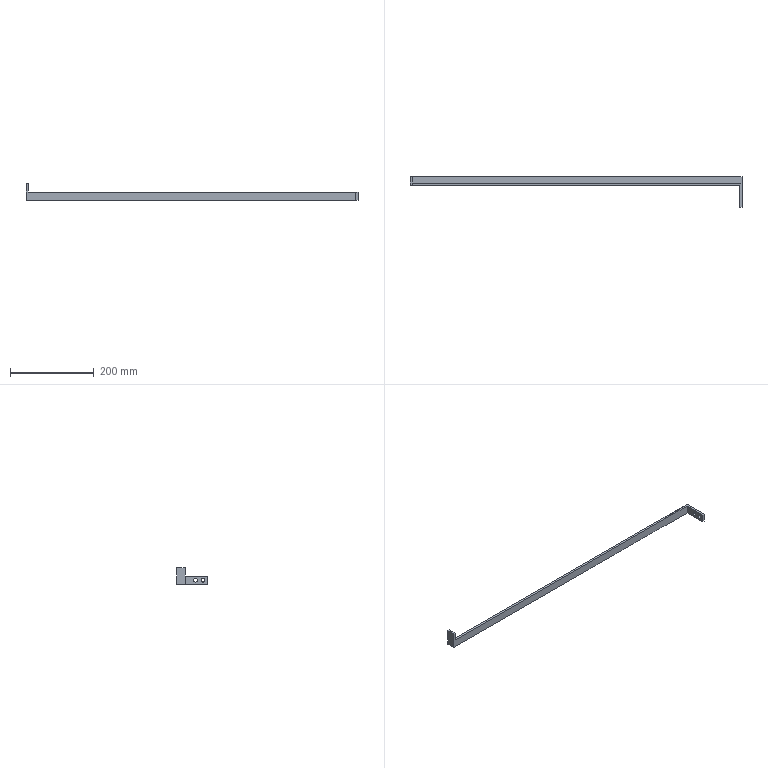Part | NX | features solid 2 | 1 solid | 14 faces | box 794.5 x 73 x 40 mm | volume 146826 mm3 | plane 12 | cylinder 2 | commonest cylinder face diameters 9 x2
STEP:
#1=CARTESIAN_POINT('',(-600.,-329.5,356.5));
#2=VERTEX_POINT('',#1);
#3=CARTESIAN_POINT('',(-600.,-276.5,356.5));
#4=VERTEX_POINT('',#3);
#5=CARTESIAN_POINT('',(-600.,-311.5,356.5));
#6=DIRECTION('',(0.,-1.,0.));
#7=VECTOR('',#6,1000.);
#8=LINE('',#5,#7);
#9=EDGE_CURVE('',#2,#4,#8,.F.);
#10=ORIENTED_EDGE('',*,*,#9,.T.);
#11=CARTESIAN_POINT('',(-1389.5,-276.5,356.5));
#12=VERTEX_POINT('',#11);
#13=CARTESIAN_POINT('',(-487.,-276.5,356.5));
#14=DIRECTION('',(-1.,0.,0.));
#15=VECTOR('',#14,1000.);
#16=LINE('',#13,#15);
#17=EDGE_CURVE('',#4,#12,#16,.T.);
#18=ORIENTED_EDGE('',*,*,#17,.T.);
#19=CARTESIAN_POINT('',(-1389.5,-256.5,356.5));
#20=VERTEX_POINT('',#19);
#21=CARTESIAN_POINT('',(-1389.5,-316.5,356.5));
#22=DIRECTION('',(0.,1.,0.));
#23=VECTOR('',#22,1000.);
#24=LINE('',#21,#23);
#25=EDGE_CURVE('',#12,#20,#24,.T.);
#26=ORIENTED_EDGE('',*,*,#25,.T.);
#27=CARTESIAN_POINT('',(-595.,-256.5,356.5));
#28=VERTEX_POINT('',#27);
#29=CARTESIAN_POINT('',(-695.5,-256.5,356.5));
#30=DIRECTION('',(1.,0.,0.));
#31=VECTOR('',#30,1000.);
#32=LINE('',#29,#31);
#33=EDGE_CURVE('',#20,#28,#32,.T.);
#34=ORIENTED_EDGE('',*,*,#33,.T.);
#35=CARTESIAN_POINT('',(-595.,-329.5,356.5));
#36=VERTEX_POINT('',#35);
#37=CARTESIAN_POINT('',(-595.,-311.5,356.5));
#38=DIRECTION('',(0.,1.,0.));
#39=VECTOR('',#38,1000.);
#40=LINE('',#37,#39);
#41=EDGE_CURVE('',#36,#28,#40,.T.);
#42=ORIENTED_EDGE('',*,*,#41,.F.);
#43=CARTESIAN_POINT('',(-595.,-329.5,356.5));
#44=DIRECTION('',(-1.,0.,0.));
#45=VECTOR('',#44,1000.);
#46=LINE('',#43,#45);
#47=EDGE_CURVE('',#36,#2,#46,.T.);
#48=ORIENTED_EDGE('',*,*,#47,.T.);
#49=EDGE_LOOP('',(#10,#18,#26,#34,#42,#48));
#50=FACE_BOUND('',#49,.T.);
#51=CARTESIAN_POINT('',(-487.,-316.5,356.5));
#52=DIRECTION('',(0.,0.,-1.));
#53=DIRECTION('',(0.,1.,0.));
#54=AXIS2_PLACEMENT_3D('',#51,#52,#53);
#55=PLANE('',#54);
#56=ADVANCED_FACE('',(#50),#55,.T.);
#57=CARTESIAN_POINT('',(-1384.5,-276.5,376.5));
#58=VERTEX_POINT('',#57);
#59=CARTESIAN_POINT('',(-600.,-276.5,376.5));
#60=VERTEX_POINT('',#59);
#61=CARTESIAN_POINT('',(-487.,-276.5,376.5));
#62=DIRECTION('',(-1.,0.,0.));
#63=VECTOR('',#62,1000.);
#64=LINE('',#61,#63);
#65=EDGE_CURVE('',#58,#60,#64,.F.);
#66=ORIENTED_EDGE('',*,*,#65,.T.);
#67=CARTESIAN_POINT('',(-600.,-329.5,376.5));
#68=VERTEX_POINT('',#67);
#69=CARTESIAN_POINT('',(-600.,-311.5,376.5));
#70=DIRECTION('',(0.,-1.,0.));
#71=VECTOR('',#70,1000.);
#72=LINE('',#69,#71);
#73=EDGE_CURVE('',#68,#60,#72,.F.);
#74=ORIENTED_EDGE('',*,*,#73,.F.);
#75=CARTESIAN_POINT('',(-595.,-329.5,376.5));
#76=VERTEX_POINT('',#75);
#77=CARTESIAN_POINT('',(-595.,-329.5,376.5));
#78=DIRECTION('',(1.,0.,0.));
#79=VECTOR('',#78,1000.);
#80=LINE('',#77,#79);
#81=EDGE_CURVE('',#76,#68,#80,.F.);
#82=ORIENTED_EDGE('',*,*,#81,.F.);
#83=CARTESIAN_POINT('',(-595.,-271.5,376.5));
#84=VERTEX_POINT('',#83);
#85=CARTESIAN_POINT('',(-595.,-316.5,376.5));
#86=DIRECTION('',(0.,-1.,0.));
#87=VECTOR('',#86,1000.);
#88=LINE('',#85,#87);
#89=EDGE_CURVE('',#76,#84,#88,.F.);
#90=ORIENTED_EDGE('',*,*,#89,.T.);
#91=CARTESIAN_POINT('',(-1384.5,-271.5,376.5));
#92=VERTEX_POINT('',#91);
#93=CARTESIAN_POINT('',(-487.,-271.5,376.5));
#94=DIRECTION('',(-1.,0.,0.));
#95=VECTOR('',#94,1000.);
#96=LINE('',#93,#95);
#97=EDGE_CURVE('',#92,#84,#96,.F.);
#98=ORIENTED_EDGE('',*,*,#97,.F.);
#99=CARTESIAN_POINT('',(-1384.5,-316.5,376.5));
#100=DIRECTION('',(0.,-1.,0.));
#101=VECTOR('',#100,1000.);
#102=LINE('',#99,#101);
#103=EDGE_CURVE('',#58,#92,#102,.F.);
#104=ORIENTED_EDGE('',*,*,#103,.F.);
#105=EDGE_LOOP('',(#66,#74,#82,#90,#98,#104));
#106=FACE_BOUND('',#105,.T.);
#107=CARTESIAN_POINT('',(-487.,-316.5,376.5));
#108=DIRECTION('',(0.,0.,-1.));
#109=DIRECTION('',(0.,1.,0.));
#110=AXIS2_PLACEMENT_3D('',#107,#108,#109);
#111=PLANE('',#110);
#112=ADVANCED_FACE('',(#106),#111,.F.);
#113=ORIENTED_EDGE('',*,*,#41,.T.);
#114=CARTESIAN_POINT('',(-595.,-256.5,361.5));
#115=VERTEX_POINT('',#114);
#116=CARTESIAN_POINT('',(-595.,-256.5,361.5));
#117=DIRECTION('',(0.,0.,1.));
#118=VECTOR('',#117,1000.);
#119=LINE('',#116,#118);
#120=EDGE_CURVE('',#28,#115,#119,.T.);
#121=ORIENTED_EDGE('',*,*,#120,.T.);
#122=CARTESIAN_POINT('',(-595.,-271.5,361.5));
#123=VERTEX_POINT('',#122);
#124=CARTESIAN_POINT('',(-595.,-311.5,361.5));
#125=DIRECTION('',(0.,1.,0.));
#126=VECTOR('',#125,1000.);
#127=LINE('',#124,#126);
#128=EDGE_CURVE('',#123,#115,#127,.T.);
#129=ORIENTED_EDGE('',*,*,#128,.F.);
#130=CARTESIAN_POINT('',(-595.,-271.5,331.));
#131=DIRECTION('',(0.,0.,1.));
#132=VECTOR('',#131,1000.);
#133=LINE('',#130,#132);
#134=EDGE_CURVE('',#123,#84,#133,.T.);
#135=ORIENTED_EDGE('',*,*,#134,.T.);
#136=ORIENTED_EDGE('',*,*,#89,.F.);
#137=CARTESIAN_POINT('',(-595.,-329.5,376.5));
#138=DIRECTION('',(0.,0.,-1.));
#139=VECTOR('',#138,1000.);
#140=LINE('',#137,#139);
#141=EDGE_CURVE('',#76,#36,#140,.T.);
#142=ORIENTED_EDGE('',*,*,#141,.T.);
#143=EDGE_LOOP('',(#113,#121,#129,#135,#136,#142));
#144=FACE_BOUND('',#143,.T.);
#145=CARTESIAN_POINT('',(-595.,-306.,366.5));
#146=VERTEX_POINT('',#145);
#147=CARTESIAN_POINT('',(-595.,-301.5,366.5));
#148=DIRECTION('',(1.,0.,0.));
#149=DIRECTION('',(0.,-1.,0.));
#150=AXIS2_PLACEMENT_3D('',#147,#148,#149);
#151=CIRCLE('',#150,4.5);
#152=EDGE_CURVE('',#146,#146,#151,.T.);
#153=ORIENTED_EDGE('',*,*,#152,.F.);
#154=EDGE_LOOP('',(#153));
#155=FACE_BOUND('',#154,.T.);
#156=CARTESIAN_POINT('',(-595.,-324.,366.5));
#157=VERTEX_POINT('',#156);
#158=CARTESIAN_POINT('',(-595.,-319.5,366.5));
#159=DIRECTION('',(1.,0.,0.));
#160=DIRECTION('',(0.,-1.,0.));
#161=AXIS2_PLACEMENT_3D('',#158,#159,#160);
#162=CIRCLE('',#161,4.5);
#163=EDGE_CURVE('',#157,#157,#162,.T.);
#164=ORIENTED_EDGE('',*,*,#163,.F.);
#165=EDGE_LOOP('',(#164));
#166=FACE_BOUND('',#165,.T.);
#167=CARTESIAN_POINT('',(-595.,-311.5,331.));
#168=DIRECTION('',(-1.,0.,0.));
#169=DIRECTION('',(0.,-1.,0.));
#170=AXIS2_PLACEMENT_3D('',#167,#168,#169);
#171=PLANE('',#170);
#172=ADVANCED_FACE('',(#144,#155,#166),#171,.F.);
#173=CARTESIAN_POINT('',(-1389.5,-256.5,396.5));
#174=VERTEX_POINT('',#173);
#175=CARTESIAN_POINT('',(-1389.5,-256.5,110.5));
#176=DIRECTION('',(0.,0.,1.));
#177=VECTOR('',#176,1000.);
#178=LINE('',#175,#177);
#179=EDGE_CURVE('',#20,#174,#178,.T.);
#180=ORIENTED_EDGE('',*,*,#179,.T.);
#181=CARTESIAN_POINT('',(-1384.5,-256.5,396.5));
#182=VERTEX_POINT('',#181);
#183=CARTESIAN_POINT('',(-1389.5,-256.5,396.5));
#184=DIRECTION('',(1.,0.,0.));
#185=VECTOR('',#184,1000.);
#186=LINE('',#183,#185);
#187=EDGE_CURVE('',#174,#182,#186,.T.);
#188=ORIENTED_EDGE('',*,*,#187,.T.);
#189=CARTESIAN_POINT('',(-1384.5,-256.5,361.5));
#190=VERTEX_POINT('',#189);
#191=CARTESIAN_POINT('',(-1384.5,-256.5,361.5));
#192=DIRECTION('',(0.,0.,1.));
#193=VECTOR('',#192,1000.);
#194=LINE('',#191,#193);
#195=EDGE_CURVE('',#190,#182,#194,.T.);
#196=ORIENTED_EDGE('',*,*,#195,.F.);
#197=CARTESIAN_POINT('',(-695.5,-256.5,361.5));
#198=DIRECTION('',(1.,0.,0.));
#199=VECTOR('',#198,1000.);
#200=LINE('',#197,#199);
#201=EDGE_CURVE('',#190,#115,#200,.T.);
#202=ORIENTED_EDGE('',*,*,#201,.T.);
#203=ORIENTED_EDGE('',*,*,#120,.F.);
#204=ORIENTED_EDGE('',*,*,#33,.F.);
#205=EDGE_LOOP('',(#180,#188,#196,#202,#203,#204));
#206=FACE_BOUND('',#205,.T.);
#207=CARTESIAN_POINT('',(-695.5,-256.5,361.5));
#208=DIRECTION('',(0.,-1.,0.));
#209=DIRECTION('',(1.,0.,0.));
#210=AXIS2_PLACEMENT_3D('',#207,#208,#209);
#211=PLANE('',#210);
#212=ADVANCED_FACE('',(#206),#211,.F.);
#213=CARTESIAN_POINT('',(-1384.5,-271.5,361.5));
#214=VERTEX_POINT('',#213);
#215=CARTESIAN_POINT('',(-695.5,-271.5,361.5));
#216=DIRECTION('',(1.,0.,0.));
#217=VECTOR('',#216,1000.);
#218=LINE('',#215,#217);
#219=EDGE_CURVE('',#214,#123,#218,.T.);
#220=ORIENTED_EDGE('',*,*,#219,.T.);
#221=ORIENTED_EDGE('',*,*,#128,.T.);
#222=ORIENTED_EDGE('',*,*,#201,.F.);
#223=CARTESIAN_POINT('',(-1384.5,-251.5,361.5));
#224=DIRECTION('',(0.,-1.,0.));
#225=VECTOR('',#224,1000.);
#226=LINE('',#223,#225);
#227=EDGE_CURVE('',#190,#214,#226,.T.);
#228=ORIENTED_EDGE('',*,*,#227,.T.);
#229=EDGE_LOOP('',(#220,#221,#222,#228));
#230=FACE_BOUND('',#229,.T.);
#231=CARTESIAN_POINT('',(-695.5,-251.5,361.5));
#232=DIRECTION('',(0.,0.,-1.));
#233=DIRECTION('',(0.,-1.,0.));
#234=AXIS2_PLACEMENT_3D('',#231,#232,#233);
#235=PLANE('',#234);
#236=ADVANCED_FACE('',(#230),#235,.F.);
#237=ORIENTED_EDGE('',*,*,#97,.T.);
#238=ORIENTED_EDGE('',*,*,#134,.F.);
#239=ORIENTED_EDGE('',*,*,#219,.F.);
#240=CARTESIAN_POINT('',(-1384.5,-271.5,381.5));
#241=DIRECTION('',(0.,0.,-1.));
#242=VECTOR('',#241,1000.);
#243=LINE('',#240,#242);
#244=EDGE_CURVE('',#92,#214,#243,.T.);
#245=ORIENTED_EDGE('',*,*,#244,.F.);
#246=EDGE_LOOP('',(#237,#238,#239,#245));
#247=FACE_BOUND('',#246,.T.);
#248=CARTESIAN_POINT('',(-695.5,-271.5,381.5));
#249=DIRECTION('',(0.,1.,0.));
#250=DIRECTION('',(0.,0.,-1.));
#251=AXIS2_PLACEMENT_3D('',#248,#249,#250);
#252=PLANE('',#251);
#253=ADVANCED_FACE('',(#247),#252,.T.);
#254=ORIENTED_EDGE('',*,*,#17,.F.);
#255=CARTESIAN_POINT('',(-600.,-276.5,381.5));
#256=DIRECTION('',(0.,0.,1.));
#257=VECTOR('',#256,1000.);
#258=LINE('',#255,#257);
#259=EDGE_CURVE('',#4,#60,#258,.T.);
#260=ORIENTED_EDGE('',*,*,#259,.T.);
#261=ORIENTED_EDGE('',*,*,#65,.F.);
#262=CARTESIAN_POINT('',(-1384.5,-276.5,396.5));
#263=VERTEX_POINT('',#262);
#264=CARTESIAN_POINT('',(-1384.5,-276.5,366.5));
#265=DIRECTION('',(0.,0.,-1.));
#266=VECTOR('',#265,1000.);
#267=LINE('',#264,#266);
#268=EDGE_CURVE('',#58,#263,#267,.F.);
#269=ORIENTED_EDGE('',*,*,#268,.T.);
#270=CARTESIAN_POINT('',(-1389.5,-276.5,396.5));
#271=VERTEX_POINT('',#270);
#272=CARTESIAN_POINT('',(-1389.5,-276.5,396.5));
#273=DIRECTION('',(1.,0.,0.));
#274=VECTOR('',#273,1000.);
#275=LINE('',#272,#274);
#276=EDGE_CURVE('',#271,#263,#275,.T.);
#277=ORIENTED_EDGE('',*,*,#276,.F.);
#278=CARTESIAN_POINT('',(-1389.5,-276.5,381.5));
#279=DIRECTION('',(0.,0.,1.));
#280=VECTOR('',#279,1000.);
#281=LINE('',#278,#280);
#282=EDGE_CURVE('',#12,#271,#281,.T.);
#283=ORIENTED_EDGE('',*,*,#282,.F.);
#284=EDGE_LOOP('',(#254,#260,#261,#269,#277,#283));
#285=FACE_BOUND('',#284,.T.);
#286=CARTESIAN_POINT('',(-695.5,-276.5,381.5));
#287=DIRECTION('',(0.,1.,0.));
#288=DIRECTION('',(0.,0.,-1.));
#289=AXIS2_PLACEMENT_3D('',#286,#287,#288);
#290=PLANE('',#289);
#291=ADVANCED_FACE('',(#285),#290,.F.);
#292=ORIENTED_EDGE('',*,*,#195,.T.);
#293=CARTESIAN_POINT('',(-1384.5,-276.5,396.5));
#294=DIRECTION('',(0.,1.,0.));
#295=VECTOR('',#294,1000.);
#296=LINE('',#293,#295);
#297=EDGE_CURVE('',#263,#182,#296,.T.);
#298=ORIENTED_EDGE('',*,*,#297,.F.);
#299=ORIENTED_EDGE('',*,*,#268,.F.);
#300=ORIENTED_EDGE('',*,*,#103,.T.);
#301=ORIENTED_EDGE('',*,*,#244,.T.);
#302=ORIENTED_EDGE('',*,*,#227,.F.);
#303=EDGE_LOOP('',(#292,#298,#299,#300,#301,#302));
#304=FACE_BOUND('',#303,.T.);
#305=CARTESIAN_POINT('',(-1384.5,-276.5,356.5));
#306=DIRECTION('',(1.,0.,0.));
#307=DIRECTION('',(0.,0.,1.));
#308=AXIS2_PLACEMENT_3D('',#305,#306,#307);
#309=PLANE('',#308);
#310=ADVANCED_FACE('',(#304),#309,.T.);
#311=ORIENTED_EDGE('',*,*,#282,.T.);
#312=CARTESIAN_POINT('',(-1389.5,-276.5,396.5));
#313=DIRECTION('',(0.,1.,0.));
#314=VECTOR('',#313,1000.);
#315=LINE('',#312,#314);
#316=EDGE_CURVE('',#271,#174,#315,.T.);
#317=ORIENTED_EDGE('',*,*,#316,.T.);
#318=ORIENTED_EDGE('',*,*,#179,.F.);
#319=ORIENTED_EDGE('',*,*,#25,.F.);
#320=EDGE_LOOP('',(#311,#317,#318,#319));
#321=FACE_BOUND('',#320,.T.);
#322=CARTESIAN_POINT('',(-1389.5,-149.5,110.5));
#323=DIRECTION('',(-1.,0.,0.));
#324=DIRECTION('',(0.,-1.,0.));
#325=AXIS2_PLACEMENT_3D('',#322,#323,#324);
#326=PLANE('',#325);
#327=ADVANCED_FACE('',(#321),#326,.T.);
#328=ORIENTED_EDGE('',*,*,#187,.F.);
#329=ORIENTED_EDGE('',*,*,#316,.F.);
#330=ORIENTED_EDGE('',*,*,#276,.T.);
#331=ORIENTED_EDGE('',*,*,#297,.T.);
#332=EDGE_LOOP('',(#328,#329,#330,#331));
#333=FACE_BOUND('',#332,.T.);
#334=CARTESIAN_POINT('',(-1389.5,-276.5,396.5));
#335=DIRECTION('',(0.,0.,-1.));
#336=DIRECTION('',(0.,1.,0.));
#337=AXIS2_PLACEMENT_3D('',#334,#335,#336);
#338=PLANE('',#337);
#339=ADVANCED_FACE('',(#333),#338,.F.);
#340=CARTESIAN_POINT('',(-600.,-297.,366.5));
#341=VERTEX_POINT('',#340);
#342=CARTESIAN_POINT('',(-600.,-301.5,366.5));
#343=DIRECTION('',(-1.,0.,0.));
#344=DIRECTION('',(0.,1.,0.));
#345=AXIS2_PLACEMENT_3D('',#342,#343,#344);
#346=CIRCLE('',#345,4.5);
#347=EDGE_CURVE('',#341,#341,#346,.T.);
#348=ORIENTED_EDGE('',*,*,#347,.F.);
#349=EDGE_LOOP('',(#348));
#350=FACE_BOUND('',#349,.T.);
#351=CARTESIAN_POINT('',(-600.,-315.,366.5));
#352=VERTEX_POINT('',#351);
#353=CARTESIAN_POINT('',(-600.,-319.5,366.5));
#354=DIRECTION('',(-1.,0.,0.));
#355=DIRECTION('',(0.,1.,0.));
#356=AXIS2_PLACEMENT_3D('',#353,#354,#355);
#357=CIRCLE('',#356,4.5);
#358=EDGE_CURVE('',#352,#352,#357,.T.);
#359=ORIENTED_EDGE('',*,*,#358,.F.);
#360=EDGE_LOOP('',(#359));
#361=FACE_BOUND('',#360,.T.);
#362=ORIENTED_EDGE('',*,*,#259,.F.);
#363=ORIENTED_EDGE('',*,*,#9,.F.);
#364=CARTESIAN_POINT('',(-600.,-329.5,376.5));
#365=DIRECTION('',(0.,0.,-1.));
#366=VECTOR('',#365,1000.);
#367=LINE('',#364,#366);
#368=EDGE_CURVE('',#68,#2,#367,.T.);
#369=ORIENTED_EDGE('',*,*,#368,.F.);
#370=ORIENTED_EDGE('',*,*,#73,.T.);
#371=EDGE_LOOP('',(#362,#363,#369,#370));
#372=FACE_BOUND('',#371,.T.);
#373=CARTESIAN_POINT('',(-600.,-311.5,376.5));
#374=DIRECTION('',(-1.,0.,0.));
#375=DIRECTION('',(0.,-1.,0.));
#376=AXIS2_PLACEMENT_3D('',#373,#374,#375);
#377=PLANE('',#376);
#378=ADVANCED_FACE('',(#350,#361,#372),#377,.T.);
#379=ORIENTED_EDGE('',*,*,#81,.T.);
#380=ORIENTED_EDGE('',*,*,#368,.T.);
#381=ORIENTED_EDGE('',*,*,#47,.F.);
#382=ORIENTED_EDGE('',*,*,#141,.F.);
#383=EDGE_LOOP('',(#379,#380,#381,#382));
#384=FACE_BOUND('',#383,.T.);
#385=CARTESIAN_POINT('',(-595.,-329.5,376.5));
#386=DIRECTION('',(0.,-1.,0.));
#387=DIRECTION('',(0.,0.,-1.));
#388=AXIS2_PLACEMENT_3D('',#385,#386,#387);
#389=PLANE('',#388);
#390=ADVANCED_FACE('',(#384),#389,.T.);
#391=ORIENTED_EDGE('',*,*,#347,.T.);
#392=EDGE_LOOP('',(#391));
#393=FACE_BOUND('',#392,.T.);
#394=ORIENTED_EDGE('',*,*,#152,.T.);
#395=EDGE_LOOP('',(#394));
#396=FACE_BOUND('',#395,.T.);
#397=CARTESIAN_POINT('',(-600.,-301.5,366.5));
#398=DIRECTION('',(1.,0.,0.));
#399=DIRECTION('',(0.,1.,0.));
#400=AXIS2_PLACEMENT_3D('',#397,#398,#399);
#401=CYLINDRICAL_SURFACE('',#400,4.5);
#402=ADVANCED_FACE('',(#393,#396),#401,.F.);
#403=ORIENTED_EDGE('',*,*,#358,.T.);
#404=EDGE_LOOP('',(#403));
#405=FACE_BOUND('',#404,.T.);
#406=ORIENTED_EDGE('',*,*,#163,.T.);
#407=EDGE_LOOP('',(#406));
#408=FACE_BOUND('',#407,.T.);
#409=CARTESIAN_POINT('',(-600.,-319.5,366.5));
#410=DIRECTION('',(1.,0.,0.));
#411=DIRECTION('',(0.,1.,0.));
#412=AXIS2_PLACEMENT_3D('',#409,#410,#411);
#413=CYLINDRICAL_SURFACE('',#412,4.5);
#414=ADVANCED_FACE('',(#405,#408),#413,.F.);
#415=CLOSED_SHELL('',(#56,#112,#172,#212,#236,#253,#291,#310,#327,#339,#378,#390,#402,#414));
#416=MANIFOLD_SOLID_BREP('',#415);
#417=(LENGTH_UNIT()NAMED_UNIT(*)SI_UNIT(.MILLI.,.METRE.));
#418=UNCERTAINTY_MEASURE_WITH_UNIT(LENGTH_MEASURE(0.00001),#417,'','');
#419=(NAMED_UNIT(*)PLANE_ANGLE_UNIT()SI_UNIT($,.RADIAN.));
#420=(NAMED_UNIT(*)SI_UNIT($,.STERADIAN.)SOLID_ANGLE_UNIT());
#421=(GEOMETRIC_REPRESENTATION_CONTEXT(3)GLOBAL_UNCERTAINTY_ASSIGNED_CONTEXT((#418))GLOBAL_UNIT_ASSIGNED_CONTEXT((#417,#419,#420))REPRESENTATION_CONTEXT('',''));
#422=ADVANCED_BREP_SHAPE_REPRESENTATION('',(#416),#421);